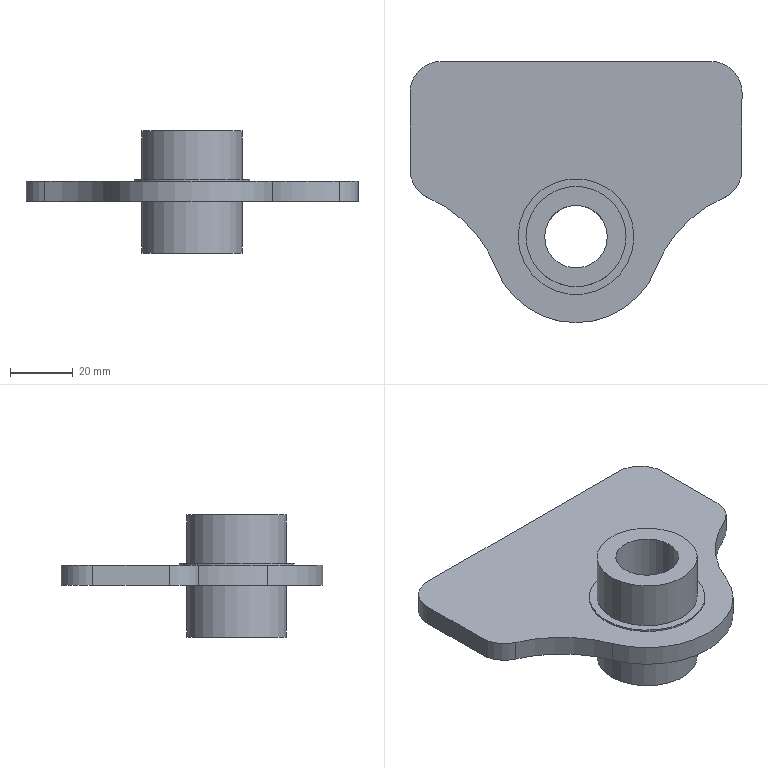Part | NX | 1 solid | 19 faces | box 106 x 83.448 x 39 mm | volume 57546 mm3 | cylinder 11 | plane 8 | commonest cylinder face diameters 20 x5 32 x2 80 x2 37 x1 55 x1
STEP:
#1=CARTESIAN_POINT('',(-18.8,6.519,-22.5));
#2=VERTEX_POINT('',#1);
#3=CARTESIAN_POINT('',(-34.8,6.519,-22.5));
#4=DIRECTION('',(0.,0.,1.));
#5=DIRECTION('',(1.,0.,0.));
#6=AXIS2_PLACEMENT_3D('',#3,#4,#5);
#7=CIRCLE('',#6,16.);
#8=EDGE_CURVE('',#2,#2,#7,.T.);
#9=ORIENTED_EDGE('',*,*,#8,.F.);
#10=EDGE_LOOP('',(#9));
#11=FACE_BOUND('',#10,.T.);
#12=CARTESIAN_POINT('',(-24.8,6.519,-22.5));
#13=VERTEX_POINT('',#12);
#14=CARTESIAN_POINT('',(-34.8,6.519,-22.5));
#15=DIRECTION('',(0.,0.,1.));
#16=DIRECTION('',(1.,0.,0.));
#17=AXIS2_PLACEMENT_3D('',#14,#15,#16);
#18=CIRCLE('',#17,10.);
#19=EDGE_CURVE('',#13,#13,#18,.T.);
#20=ORIENTED_EDGE('',*,*,#19,.T.);
#21=EDGE_LOOP('',(#20));
#22=FACE_BOUND('',#21,.T.);
#23=CARTESIAN_POINT('',(-34.8,6.519,-22.5));
#24=DIRECTION('',(0.,0.,1.));
#25=DIRECTION('',(1.,0.,0.));
#26=AXIS2_PLACEMENT_3D('',#23,#24,#25);
#27=PLANE('',#26);
#28=ADVANCED_FACE('',(#11,#22),#27,.F.);
#29=CARTESIAN_POINT('',(-18.8,6.519,-6.));
#30=VERTEX_POINT('',#29);
#31=CARTESIAN_POINT('',(-34.8,6.519,-6.));
#32=DIRECTION('',(0.,0.,1.));
#33=DIRECTION('',(1.,0.,0.));
#34=AXIS2_PLACEMENT_3D('',#31,#32,#33);
#35=CIRCLE('',#34,16.);
#36=EDGE_CURVE('',#30,#30,#35,.T.);
#37=ORIENTED_EDGE('',*,*,#36,.T.);
#38=EDGE_LOOP('',(#37));
#39=FACE_BOUND('',#38,.T.);
#40=CARTESIAN_POINT('',(-60.431,-3.391,-6.));
#41=VERTEX_POINT('',#40);
#42=CARTESIAN_POINT('',(-9.167,-3.39,-6.));
#43=VERTEX_POINT('',#42);
#44=CARTESIAN_POINT('',(-34.799,6.571,-6.));
#45=DIRECTION('',(0.,0.,1.));
#46=DIRECTION('',(1.,0.,0.));
#47=AXIS2_PLACEMENT_3D('',#44,#45,#46);
#48=CIRCLE('',#47,27.5);
#49=EDGE_CURVE('',#41,#43,#48,.T.);
#50=ORIENTED_EDGE('',*,*,#49,.F.);
#51=CARTESIAN_POINT('',(-81.783,18.81,-6.));
#52=VERTEX_POINT('',#51);
#53=CARTESIAN_POINT('',(-97.715,-17.881,-6.));
#54=DIRECTION('',(0.,0.,-1.));
#55=DIRECTION('',(1.,0.,0.));
#56=AXIS2_PLACEMENT_3D('',#53,#54,#55);
#57=CIRCLE('',#56,40.);
#58=EDGE_CURVE('',#52,#41,#57,.T.);
#59=ORIENTED_EDGE('',*,*,#58,.F.);
#60=CARTESIAN_POINT('',(-87.8,27.982,-6.));
#61=VERTEX_POINT('',#60);
#62=CARTESIAN_POINT('',(-77.8,27.982,-6.));
#63=DIRECTION('',(0.,0.,1.));
#64=DIRECTION('',(1.,0.,0.));
#65=AXIS2_PLACEMENT_3D('',#62,#63,#64);
#66=CIRCLE('',#65,10.);
#67=EDGE_CURVE('',#61,#52,#66,.T.);
#68=ORIENTED_EDGE('',*,*,#67,.F.);
#69=CARTESIAN_POINT('',(-87.8,52.519,-6.));
#70=VERTEX_POINT('',#69);
#71=CARTESIAN_POINT('',(-87.8,52.519,-6.));
#72=DIRECTION('',(0.,-1.,0.));
#73=VECTOR('',#72,1000.);
#74=LINE('',#71,#73);
#75=EDGE_CURVE('',#70,#61,#74,.T.);
#76=ORIENTED_EDGE('',*,*,#75,.F.);
#77=CARTESIAN_POINT('',(-77.8,62.519,-6.));
#78=VERTEX_POINT('',#77);
#79=CARTESIAN_POINT('',(-77.8,52.519,-6.));
#80=DIRECTION('',(0.,0.,1.));
#81=DIRECTION('',(1.,0.,0.));
#82=AXIS2_PLACEMENT_3D('',#79,#80,#81);
#83=CIRCLE('',#82,10.);
#84=EDGE_CURVE('',#78,#70,#83,.T.);
#85=ORIENTED_EDGE('',*,*,#84,.F.);
#86=CARTESIAN_POINT('',(8.2,62.519,-6.));
#87=VERTEX_POINT('',#86);
#88=CARTESIAN_POINT('',(5.2,62.519,-6.));
#89=DIRECTION('',(-1.,0.,0.));
#90=VECTOR('',#89,1000.);
#91=LINE('',#88,#90);
#92=EDGE_CURVE('',#87,#78,#91,.T.);
#93=ORIENTED_EDGE('',*,*,#92,.F.);
#94=CARTESIAN_POINT('',(18.2,52.519,-6.));
#95=VERTEX_POINT('',#94);
#96=CARTESIAN_POINT('',(8.2,52.519,-6.));
#97=DIRECTION('',(0.,0.,1.));
#98=DIRECTION('',(1.,0.,0.));
#99=AXIS2_PLACEMENT_3D('',#96,#97,#98);
#100=CIRCLE('',#99,10.);
#101=EDGE_CURVE('',#95,#87,#100,.T.);
#102=ORIENTED_EDGE('',*,*,#101,.F.);
#103=CARTESIAN_POINT('',(18.2,27.982,-6.));
#104=VERTEX_POINT('',#103);
#105=CARTESIAN_POINT('',(18.2,27.982,-6.));
#106=DIRECTION('',(0.,1.,0.));
#107=VECTOR('',#106,1000.);
#108=LINE('',#105,#107);
#109=EDGE_CURVE('',#104,#95,#108,.T.);
#110=ORIENTED_EDGE('',*,*,#109,.F.);
#111=CARTESIAN_POINT('',(12.184,18.81,-6.));
#112=VERTEX_POINT('',#111);
#113=CARTESIAN_POINT('',(8.2,27.982,-6.));
#114=DIRECTION('',(0.,0.,1.));
#115=DIRECTION('',(1.,0.,0.));
#116=AXIS2_PLACEMENT_3D('',#113,#114,#115);
#117=CIRCLE('',#116,10.);
#118=EDGE_CURVE('',#112,#104,#117,.T.);
#119=ORIENTED_EDGE('',*,*,#118,.F.);
#120=CARTESIAN_POINT('',(28.116,-17.88,-6.));
#121=DIRECTION('',(0.,0.,-1.));
#122=DIRECTION('',(1.,0.,0.));
#123=AXIS2_PLACEMENT_3D('',#120,#121,#122);
#124=CIRCLE('',#123,40.);
#125=EDGE_CURVE('',#43,#112,#124,.T.);
#126=ORIENTED_EDGE('',*,*,#125,.F.);
#127=EDGE_LOOP('',(#50,#59,#68,#76,#85,#93,#102,#110,#119,#126));
#128=FACE_BOUND('',#127,.T.);
#129=CARTESIAN_POINT('',(-34.8,6.519,-6.));
#130=DIRECTION('',(0.,0.,1.));
#131=DIRECTION('',(1.,0.,0.));
#132=AXIS2_PLACEMENT_3D('',#129,#130,#131);
#133=PLANE('',#132);
#134=ADVANCED_FACE('',(#39,#128),#133,.F.);
#135=CARTESIAN_POINT('',(-60.431,-3.391,0.5));
#136=VERTEX_POINT('',#135);
#137=CARTESIAN_POINT('',(-9.167,-3.39,0.5));
#138=VERTEX_POINT('',#137);
#139=CARTESIAN_POINT('',(-34.799,6.571,0.5));
#140=DIRECTION('',(0.,0.,1.));
#141=DIRECTION('',(1.,0.,0.));
#142=AXIS2_PLACEMENT_3D('',#139,#140,#141);
#143=CIRCLE('',#142,27.5);
#144=EDGE_CURVE('',#136,#138,#143,.T.);
#145=ORIENTED_EDGE('',*,*,#144,.F.);
#146=CARTESIAN_POINT('',(-60.431,-3.391,-6.));
#147=DIRECTION('',(0.,0.,1.));
#148=VECTOR('',#147,1000.);
#149=LINE('',#146,#148);
#150=EDGE_CURVE('',#41,#136,#149,.T.);
#151=ORIENTED_EDGE('',*,*,#150,.F.);
#152=ORIENTED_EDGE('',*,*,#49,.T.);
#153=CARTESIAN_POINT('',(-9.167,-3.39,-6.));
#154=DIRECTION('',(0.,0.,1.));
#155=VECTOR('',#154,1000.);
#156=LINE('',#153,#155);
#157=EDGE_CURVE('',#43,#138,#156,.T.);
#158=ORIENTED_EDGE('',*,*,#157,.T.);
#159=EDGE_LOOP('',(#145,#151,#152,#158));
#160=FACE_BOUND('',#159,.T.);
#161=CARTESIAN_POINT('',(-34.799,6.571,-6.));
#162=DIRECTION('',(0.,0.,1.));
#163=DIRECTION('',(1.,0.,0.));
#164=AXIS2_PLACEMENT_3D('',#161,#162,#163);
#165=CYLINDRICAL_SURFACE('',#164,27.5);
#166=ADVANCED_FACE('',(#160),#165,.T.);
#167=CARTESIAN_POINT('',(12.184,18.81,0.5));
#168=VERTEX_POINT('',#167);
#169=CARTESIAN_POINT('',(28.116,-17.88,0.5));
#170=DIRECTION('',(0.,0.,1.));
#171=DIRECTION('',(1.,0.,0.));
#172=AXIS2_PLACEMENT_3D('',#169,#170,#171);
#173=CIRCLE('',#172,40.);
#174=EDGE_CURVE('',#138,#168,#173,.F.);
#175=ORIENTED_EDGE('',*,*,#174,.F.);
#176=ORIENTED_EDGE('',*,*,#157,.F.);
#177=ORIENTED_EDGE('',*,*,#125,.T.);
#178=CARTESIAN_POINT('',(12.184,18.81,-6.));
#179=DIRECTION('',(0.,0.,1.));
#180=VECTOR('',#179,1000.);
#181=LINE('',#178,#180);
#182=EDGE_CURVE('',#112,#168,#181,.T.);
#183=ORIENTED_EDGE('',*,*,#182,.T.);
#184=EDGE_LOOP('',(#175,#176,#177,#183));
#185=FACE_BOUND('',#184,.T.);
#186=CARTESIAN_POINT('',(28.116,-17.88,-6.));
#187=DIRECTION('',(0.,0.,1.));
#188=DIRECTION('',(1.,0.,0.));
#189=AXIS2_PLACEMENT_3D('',#186,#187,#188);
#190=CYLINDRICAL_SURFACE('',#189,40.);
#191=ADVANCED_FACE('',(#185),#190,.F.);
#192=CARTESIAN_POINT('',(18.2,27.982,0.5));
#193=VERTEX_POINT('',#192);
#194=CARTESIAN_POINT('',(8.2,27.982,0.5));
#195=DIRECTION('',(0.,0.,1.));
#196=DIRECTION('',(1.,0.,0.));
#197=AXIS2_PLACEMENT_3D('',#194,#195,#196);
#198=CIRCLE('',#197,10.);
#199=EDGE_CURVE('',#168,#193,#198,.T.);
#200=ORIENTED_EDGE('',*,*,#199,.F.);
#201=ORIENTED_EDGE('',*,*,#182,.F.);
#202=ORIENTED_EDGE('',*,*,#118,.T.);
#203=CARTESIAN_POINT('',(18.2,27.982,-6.));
#204=DIRECTION('',(0.,0.,-1.));
#205=VECTOR('',#204,1000.);
#206=LINE('',#203,#205);
#207=EDGE_CURVE('',#104,#193,#206,.F.);
#208=ORIENTED_EDGE('',*,*,#207,.T.);
#209=EDGE_LOOP('',(#200,#201,#202,#208));
#210=FACE_BOUND('',#209,.T.);
#211=CARTESIAN_POINT('',(8.2,27.982,-6.));
#212=DIRECTION('',(0.,0.,1.));
#213=DIRECTION('',(1.,0.,0.));
#214=AXIS2_PLACEMENT_3D('',#211,#212,#213);
#215=CYLINDRICAL_SURFACE('',#214,10.);
#216=ADVANCED_FACE('',(#210),#215,.T.);
#217=CARTESIAN_POINT('',(18.2,52.519,0.5));
#218=VERTEX_POINT('',#217);
#219=CARTESIAN_POINT('',(18.2,6.519,0.5));
#220=DIRECTION('',(0.,1.,0.));
#221=VECTOR('',#220,1000.);
#222=LINE('',#219,#221);
#223=EDGE_CURVE('',#193,#218,#222,.T.);
#224=ORIENTED_EDGE('',*,*,#223,.F.);
#225=ORIENTED_EDGE('',*,*,#207,.F.);
#226=ORIENTED_EDGE('',*,*,#109,.T.);
#227=CARTESIAN_POINT('',(18.2,52.519,-6.));
#228=DIRECTION('',(0.,0.,1.));
#229=VECTOR('',#228,1000.);
#230=LINE('',#227,#229);
#231=EDGE_CURVE('',#95,#218,#230,.T.);
#232=ORIENTED_EDGE('',*,*,#231,.T.);
#233=EDGE_LOOP('',(#224,#225,#226,#232));
#234=FACE_BOUND('',#233,.T.);
#235=CARTESIAN_POINT('',(18.2,51.519,-6.));
#236=DIRECTION('',(1.,0.,0.));
#237=DIRECTION('',(0.,1.,0.));
#238=AXIS2_PLACEMENT_3D('',#235,#236,#237);
#239=PLANE('',#238);
#240=ADVANCED_FACE('',(#234),#239,.T.);
#241=CARTESIAN_POINT('',(8.2,62.519,0.5));
#242=VERTEX_POINT('',#241);
#243=CARTESIAN_POINT('',(8.2,52.519,0.5));
#244=DIRECTION('',(0.,0.,1.));
#245=DIRECTION('',(1.,0.,0.));
#246=AXIS2_PLACEMENT_3D('',#243,#244,#245);
#247=CIRCLE('',#246,10.);
#248=EDGE_CURVE('',#218,#242,#247,.T.);
#249=ORIENTED_EDGE('',*,*,#248,.F.);
#250=ORIENTED_EDGE('',*,*,#231,.F.);
#251=ORIENTED_EDGE('',*,*,#101,.T.);
#252=CARTESIAN_POINT('',(8.2,62.519,-6.));
#253=DIRECTION('',(0.,0.,1.));
#254=VECTOR('',#253,1000.);
#255=LINE('',#252,#254);
#256=EDGE_CURVE('',#87,#242,#255,.T.);
#257=ORIENTED_EDGE('',*,*,#256,.T.);
#258=EDGE_LOOP('',(#249,#250,#251,#257));
#259=FACE_BOUND('',#258,.T.);
#260=CARTESIAN_POINT('',(8.2,52.519,-6.));
#261=DIRECTION('',(0.,0.,1.));
#262=DIRECTION('',(1.,0.,0.));
#263=AXIS2_PLACEMENT_3D('',#260,#261,#262);
#264=CYLINDRICAL_SURFACE('',#263,10.);
#265=ADVANCED_FACE('',(#259),#264,.T.);
#266=CARTESIAN_POINT('',(-77.8,62.519,0.5));
#267=VERTEX_POINT('',#266);
#268=CARTESIAN_POINT('',(-34.8,62.519,0.5));
#269=DIRECTION('',(-1.,0.,0.));
#270=VECTOR('',#269,1000.);
#271=LINE('',#268,#270);
#272=EDGE_CURVE('',#242,#267,#271,.T.);
#273=ORIENTED_EDGE('',*,*,#272,.F.);
#274=ORIENTED_EDGE('',*,*,#256,.F.);
#275=ORIENTED_EDGE('',*,*,#92,.T.);
#276=CARTESIAN_POINT('',(-77.8,62.519,-6.));
#277=DIRECTION('',(0.,0.,1.));
#278=VECTOR('',#277,1000.);
#279=LINE('',#276,#278);
#280=EDGE_CURVE('',#78,#267,#279,.T.);
#281=ORIENTED_EDGE('',*,*,#280,.T.);
#282=EDGE_LOOP('',(#273,#274,#275,#281));
#283=FACE_BOUND('',#282,.T.);
#284=CARTESIAN_POINT('',(5.2,62.519,-6.));
#285=DIRECTION('',(0.,1.,0.));
#286=DIRECTION('',(-1.,0.,0.));
#287=AXIS2_PLACEMENT_3D('',#284,#285,#286);
#288=PLANE('',#287);
#289=ADVANCED_FACE('',(#283),#288,.T.);
#290=CARTESIAN_POINT('',(-87.8,52.519,0.5));
#291=VERTEX_POINT('',#290);
#292=CARTESIAN_POINT('',(-77.8,52.519,0.5));
#293=DIRECTION('',(0.,0.,1.));
#294=DIRECTION('',(1.,0.,0.));
#295=AXIS2_PLACEMENT_3D('',#292,#293,#294);
#296=CIRCLE('',#295,10.);
#297=EDGE_CURVE('',#267,#291,#296,.T.);
#298=ORIENTED_EDGE('',*,*,#297,.F.);
#299=ORIENTED_EDGE('',*,*,#280,.F.);
#300=ORIENTED_EDGE('',*,*,#84,.T.);
#301=CARTESIAN_POINT('',(-87.8,52.519,-6.));
#302=DIRECTION('',(0.,0.,1.));
#303=VECTOR('',#302,1000.);
#304=LINE('',#301,#303);
#305=EDGE_CURVE('',#70,#291,#304,.T.);
#306=ORIENTED_EDGE('',*,*,#305,.T.);
#307=EDGE_LOOP('',(#298,#299,#300,#306));
#308=FACE_BOUND('',#307,.T.);
#309=CARTESIAN_POINT('',(-77.8,52.519,-6.));
#310=DIRECTION('',(0.,0.,1.));
#311=DIRECTION('',(1.,0.,0.));
#312=AXIS2_PLACEMENT_3D('',#309,#310,#311);
#313=CYLINDRICAL_SURFACE('',#312,10.);
#314=ADVANCED_FACE('',(#308),#313,.T.);
#315=CARTESIAN_POINT('',(-87.8,27.982,0.5));
#316=VERTEX_POINT('',#315);
#317=CARTESIAN_POINT('',(-87.8,6.519,0.5));
#318=DIRECTION('',(0.,-1.,0.));
#319=VECTOR('',#318,1000.);
#320=LINE('',#317,#319);
#321=EDGE_CURVE('',#291,#316,#320,.T.);
#322=ORIENTED_EDGE('',*,*,#321,.F.);
#323=ORIENTED_EDGE('',*,*,#305,.F.);
#324=ORIENTED_EDGE('',*,*,#75,.T.);
#325=CARTESIAN_POINT('',(-87.8,27.982,-6.));
#326=DIRECTION('',(0.,0.,1.));
#327=VECTOR('',#326,1000.);
#328=LINE('',#325,#327);
#329=EDGE_CURVE('',#61,#316,#328,.T.);
#330=ORIENTED_EDGE('',*,*,#329,.T.);
#331=EDGE_LOOP('',(#322,#323,#324,#330));
#332=FACE_BOUND('',#331,.T.);
#333=CARTESIAN_POINT('',(-87.8,51.519,-6.));
#334=DIRECTION('',(-1.,0.,0.));
#335=DIRECTION('',(0.,0.,1.));
#336=AXIS2_PLACEMENT_3D('',#333,#334,#335);
#337=PLANE('',#336);
#338=ADVANCED_FACE('',(#332),#337,.T.);
#339=CARTESIAN_POINT('',(-81.783,18.81,0.5));
#340=VERTEX_POINT('',#339);
#341=CARTESIAN_POINT('',(-77.8,27.982,0.5));
#342=DIRECTION('',(0.,0.,1.));
#343=DIRECTION('',(1.,0.,0.));
#344=AXIS2_PLACEMENT_3D('',#341,#342,#343);
#345=CIRCLE('',#344,10.);
#346=EDGE_CURVE('',#316,#340,#345,.T.);
#347=ORIENTED_EDGE('',*,*,#346,.F.);
#348=ORIENTED_EDGE('',*,*,#329,.F.);
#349=ORIENTED_EDGE('',*,*,#67,.T.);
#350=CARTESIAN_POINT('',(-81.783,18.81,-6.));
#351=DIRECTION('',(0.,0.,1.));
#352=VECTOR('',#351,1000.);
#353=LINE('',#350,#352);
#354=EDGE_CURVE('',#52,#340,#353,.T.);
#355=ORIENTED_EDGE('',*,*,#354,.T.);
#356=EDGE_LOOP('',(#347,#348,#349,#355));
#357=FACE_BOUND('',#356,.T.);
#358=CARTESIAN_POINT('',(-77.8,27.982,-6.));
#359=DIRECTION('',(0.,0.,1.));
#360=DIRECTION('',(1.,0.,0.));
#361=AXIS2_PLACEMENT_3D('',#358,#359,#360);
#362=CYLINDRICAL_SURFACE('',#361,10.);
#363=ADVANCED_FACE('',(#357),#362,.T.);
#364=CARTESIAN_POINT('',(-97.715,-17.881,0.5));
#365=DIRECTION('',(0.,0.,1.));
#366=DIRECTION('',(1.,0.,0.));
#367=AXIS2_PLACEMENT_3D('',#364,#365,#366);
#368=CIRCLE('',#367,40.);
#369=EDGE_CURVE('',#340,#136,#368,.F.);
#370=ORIENTED_EDGE('',*,*,#369,.F.);
#371=ORIENTED_EDGE('',*,*,#354,.F.);
#372=ORIENTED_EDGE('',*,*,#58,.T.);
#373=ORIENTED_EDGE('',*,*,#150,.T.);
#374=EDGE_LOOP('',(#370,#371,#372,#373));
#375=FACE_BOUND('',#374,.T.);
#376=CARTESIAN_POINT('',(-97.715,-17.881,-6.));
#377=DIRECTION('',(0.,0.,1.));
#378=DIRECTION('',(1.,0.,0.));
#379=AXIS2_PLACEMENT_3D('',#376,#377,#378);
#380=CYLINDRICAL_SURFACE('',#379,40.);
#381=ADVANCED_FACE('',(#375),#380,.F.);
#382=CARTESIAN_POINT('',(-16.3,6.519,0.5));
#383=VERTEX_POINT('',#382);
#384=CARTESIAN_POINT('',(-34.8,6.519,0.5));
#385=DIRECTION('',(0.,0.,1.));
#386=DIRECTION('',(1.,0.,0.));
#387=AXIS2_PLACEMENT_3D('',#384,#385,#386);
#388=CIRCLE('',#387,18.5);
#389=EDGE_CURVE('',#383,#383,#388,.T.);
#390=ORIENTED_EDGE('',*,*,#389,.F.);
#391=EDGE_LOOP('',(#390));
#392=FACE_BOUND('',#391,.T.);
#393=ORIENTED_EDGE('',*,*,#144,.T.);
#394=ORIENTED_EDGE('',*,*,#174,.T.);
#395=ORIENTED_EDGE('',*,*,#199,.T.);
#396=ORIENTED_EDGE('',*,*,#223,.T.);
#397=ORIENTED_EDGE('',*,*,#248,.T.);
#398=ORIENTED_EDGE('',*,*,#272,.T.);
#399=ORIENTED_EDGE('',*,*,#297,.T.);
#400=ORIENTED_EDGE('',*,*,#321,.T.);
#401=ORIENTED_EDGE('',*,*,#346,.T.);
#402=ORIENTED_EDGE('',*,*,#369,.T.);
#403=EDGE_LOOP('',(#393,#394,#395,#396,#397,#398,#399,#400,#401,#402));
#404=FACE_BOUND('',#403,.T.);
#405=CARTESIAN_POINT('',(-34.8,6.519,0.5));
#406=DIRECTION('',(0.,0.,1.));
#407=DIRECTION('',(1.,0.,0.));
#408=AXIS2_PLACEMENT_3D('',#405,#406,#407);
#409=PLANE('',#408);
#410=ADVANCED_FACE('',(#392,#404),#409,.T.);
#411=CARTESIAN_POINT('',(-18.8,6.519,16.5));
#412=VERTEX_POINT('',#411);
#413=CARTESIAN_POINT('',(-34.8,6.519,16.5));
#414=DIRECTION('',(0.,0.,1.));
#415=DIRECTION('',(1.,0.,0.));
#416=AXIS2_PLACEMENT_3D('',#413,#414,#415);
#417=CIRCLE('',#416,16.);
#418=EDGE_CURVE('',#412,#412,#417,.T.);
#419=ORIENTED_EDGE('',*,*,#418,.F.);
#420=EDGE_LOOP('',(#419));
#421=FACE_BOUND('',#420,.T.);
#422=CARTESIAN_POINT('',(-50.8,6.519,1.));
#423=VERTEX_POINT('',#422);
#424=CARTESIAN_POINT('',(-34.8,6.519,1.));
#425=DIRECTION('',(0.,0.,-1.));
#426=DIRECTION('',(-1.,0.,0.));
#427=AXIS2_PLACEMENT_3D('',#424,#425,#426);
#428=CIRCLE('',#427,16.);
#429=EDGE_CURVE('',#423,#423,#428,.T.);
#430=ORIENTED_EDGE('',*,*,#429,.F.);
#431=EDGE_LOOP('',(#430));
#432=FACE_BOUND('',#431,.T.);
#433=CARTESIAN_POINT('',(-34.8,6.519,16.5));
#434=DIRECTION('',(0.,0.,-1.));
#435=DIRECTION('',(-1.,0.,0.));
#436=AXIS2_PLACEMENT_3D('',#433,#434,#435);
#437=CYLINDRICAL_SURFACE('',#436,16.);
#438=ADVANCED_FACE('',(#421,#432),#437,.T.);
#439=ORIENTED_EDGE('',*,*,#19,.F.);
#440=EDGE_LOOP('',(#439));
#441=FACE_BOUND('',#440,.T.);
#442=CARTESIAN_POINT('',(-24.8,6.519,16.5));
#443=VERTEX_POINT('',#442);
#444=CARTESIAN_POINT('',(-34.8,6.519,16.5));
#445=DIRECTION('',(0.,0.,1.));
#446=DIRECTION('',(1.,0.,0.));
#447=AXIS2_PLACEMENT_3D('',#444,#445,#446);
#448=CIRCLE('',#447,10.);
#449=EDGE_CURVE('',#443,#443,#448,.T.);
#450=ORIENTED_EDGE('',*,*,#449,.T.);
#451=EDGE_LOOP('',(#450));
#452=FACE_BOUND('',#451,.T.);
#453=CARTESIAN_POINT('',(-34.8,6.519,16.5));
#454=DIRECTION('',(0.,0.,-1.));
#455=DIRECTION('',(-1.,0.,0.));
#456=AXIS2_PLACEMENT_3D('',#453,#454,#455);
#457=CYLINDRICAL_SURFACE('',#456,10.);
#458=ADVANCED_FACE('',(#441,#452),#457,.F.);
#459=ORIENTED_EDGE('',*,*,#418,.T.);
#460=EDGE_LOOP('',(#459));
#461=FACE_BOUND('',#460,.T.);
#462=ORIENTED_EDGE('',*,*,#449,.F.);
#463=EDGE_LOOP('',(#462));
#464=FACE_BOUND('',#463,.T.);
#465=CARTESIAN_POINT('',(-34.8,6.519,16.5));
#466=DIRECTION('',(0.,0.,1.));
#467=DIRECTION('',(1.,0.,0.));
#468=AXIS2_PLACEMENT_3D('',#465,#466,#467);
#469=PLANE('',#468);
#470=ADVANCED_FACE('',(#461,#464),#469,.T.);
#471=ORIENTED_EDGE('',*,*,#389,.T.);
#472=EDGE_LOOP('',(#471));
#473=FACE_BOUND('',#472,.T.);
#474=CARTESIAN_POINT('',(-16.3,6.519,1.));
#475=VERTEX_POINT('',#474);
#476=CARTESIAN_POINT('',(-34.8,6.519,1.));
#477=DIRECTION('',(0.,0.,-1.));
#478=DIRECTION('',(1.,0.,0.));
#479=AXIS2_PLACEMENT_3D('',#476,#477,#478);
#480=CIRCLE('',#479,18.5);
#481=EDGE_CURVE('',#475,#475,#480,.T.);
#482=ORIENTED_EDGE('',*,*,#481,.T.);
#483=EDGE_LOOP('',(#482));
#484=FACE_BOUND('',#483,.T.);
#485=CARTESIAN_POINT('',(-34.8,6.519,1.));
#486=DIRECTION('',(0.,0.,-1.));
#487=DIRECTION('',(-1.,0.,0.));
#488=AXIS2_PLACEMENT_3D('',#485,#486,#487);
#489=CYLINDRICAL_SURFACE('',#488,18.5);
#490=ADVANCED_FACE('',(#473,#484),#489,.T.);
#491=ORIENTED_EDGE('',*,*,#429,.T.);
#492=EDGE_LOOP('',(#491));
#493=FACE_BOUND('',#492,.T.);
#494=ORIENTED_EDGE('',*,*,#481,.F.);
#495=EDGE_LOOP('',(#494));
#496=FACE_BOUND('',#495,.T.);
#497=CARTESIAN_POINT('',(-34.8,6.519,1.));
#498=DIRECTION('',(0.,0.,-1.));
#499=DIRECTION('',(-1.,0.,0.));
#500=AXIS2_PLACEMENT_3D('',#497,#498,#499);
#501=PLANE('',#500);
#502=ADVANCED_FACE('',(#493,#496),#501,.F.);
#503=ORIENTED_EDGE('',*,*,#8,.T.);
#504=EDGE_LOOP('',(#503));
#505=FACE_BOUND('',#504,.T.);
#506=ORIENTED_EDGE('',*,*,#36,.F.);
#507=EDGE_LOOP('',(#506));
#508=FACE_BOUND('',#507,.T.);
#509=CARTESIAN_POINT('',(-34.8,6.519,-25.));
#510=DIRECTION('',(0.,0.,1.));
#511=DIRECTION('',(1.,0.,0.));
#512=AXIS2_PLACEMENT_3D('',#509,#510,#511);
#513=CYLINDRICAL_SURFACE('',#512,16.);
#514=ADVANCED_FACE('',(#505,#508),#513,.T.);
#515=CLOSED_SHELL('',(#28,#134,#166,#191,#216,#240,#265,#289,#314,#338,#363,#381,#410,#438,#458,#470,#490,#502,#514));
#516=MANIFOLD_SOLID_BREP('',#515);
#517=(LENGTH_UNIT()NAMED_UNIT(*)SI_UNIT(.MILLI.,.METRE.));
#518=UNCERTAINTY_MEASURE_WITH_UNIT(LENGTH_MEASURE(0.00001),#517,'','');
#519=(NAMED_UNIT(*)PLANE_ANGLE_UNIT()SI_UNIT($,.RADIAN.));
#520=(NAMED_UNIT(*)SI_UNIT($,.STERADIAN.)SOLID_ANGLE_UNIT());
#521=(GEOMETRIC_REPRESENTATION_CONTEXT(3)GLOBAL_UNCERTAINTY_ASSIGNED_CONTEXT((#518))GLOBAL_UNIT_ASSIGNED_CONTEXT((#517,#519,#520))REPRESENTATION_CONTEXT('',''));
#522=ADVANCED_BREP_SHAPE_REPRESENTATION('',(#516),#521);